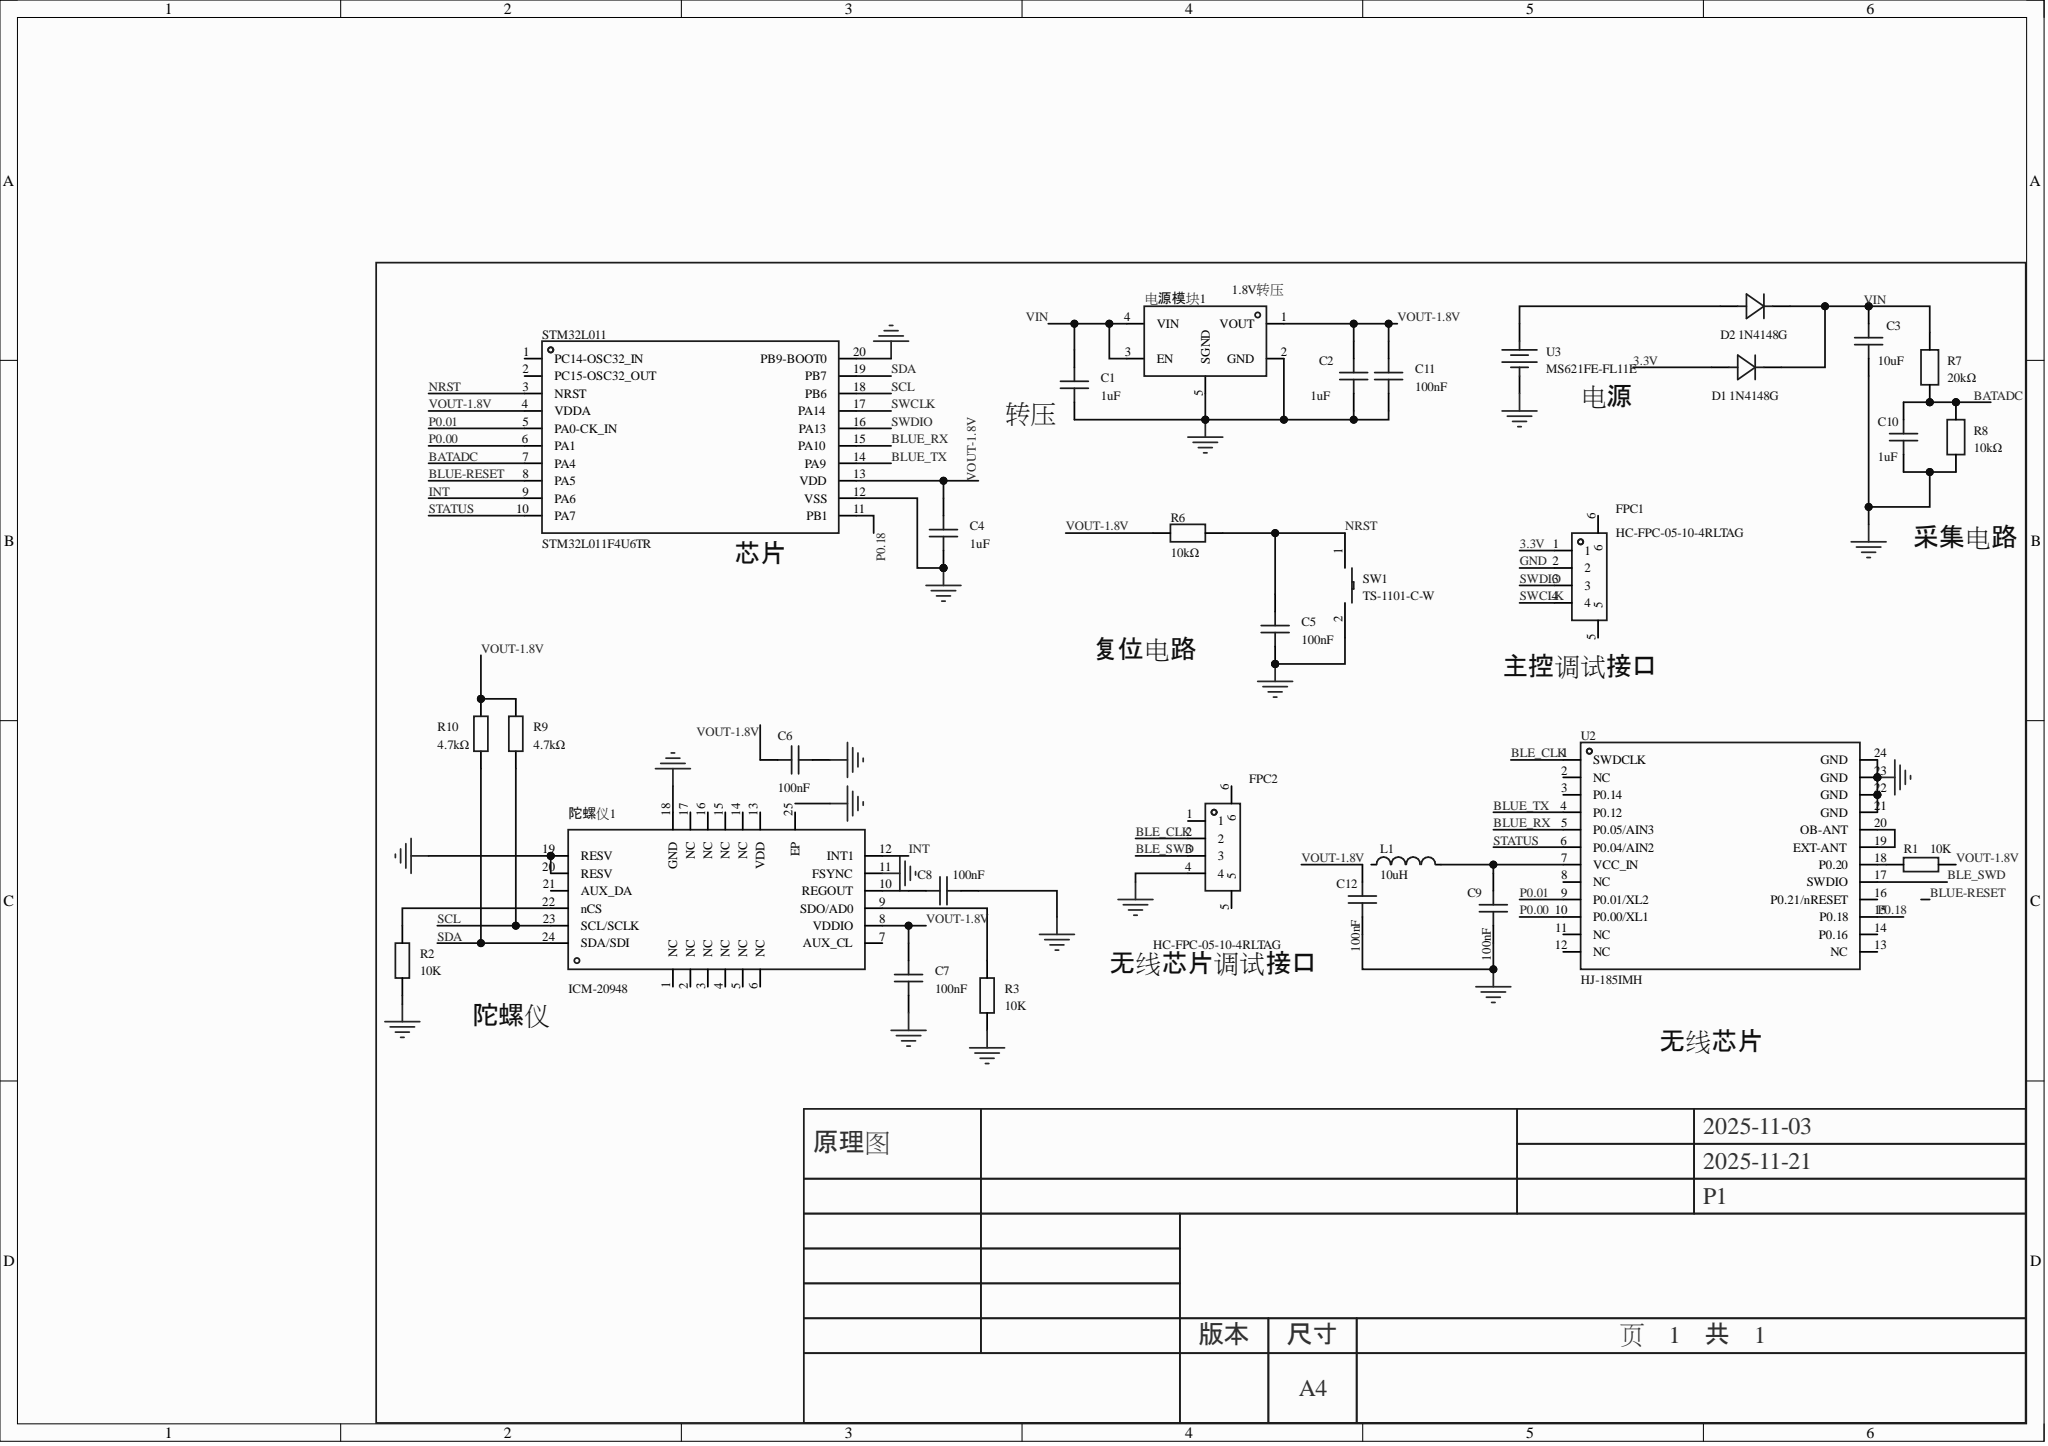Circuit board | Altium Designer | 31 parts | 26 nets
Bill of materials:
Comment,Description,Designator,Footprint,LibRef,Quantity
"1uF","容值:1uF;精度:±10%;额定电压:25V;温度系数:X5R;","C1, C2, C4, C10","C0402","CL05A105KA5NQNC","4"
"10uF","容值:10uF;精度:±10%;额定电压:50V;温度系数:X5R;","C3","C0805","CGA0805X5R106K500MT","1"
"100nF","","C5, C6, C7, C8, C9, C12","C0402","CL05B104KB54PNC, CL05B104KO5NNNC","6"
"100nF","容值:100nF;精度:±10%;额定电压:50V;温度系数:X7R;","C11","C0603","CGA0603X7R104K500JT","1"
"1N4148G","正向压降(Vf):1.25V@150mA;直流反向耐压(Vr):100V;整流电流:150mA;反向恢复时间(Trr):4ns;","D1, D2","SOD-723_L1.0-W0.6-P1.4-RD","1N4148G","2"
"HC-FPC-05-10-4RLTAG","锁定特性:翻盖式;触点类型:下接;触点数量:4P;间距:0.5mm;安装方式:卧贴;工作温度:-55℃~+85℃;","FPC1, FPC2","FPC-SMD_4P-P0.50_HCTL_HC-FPC-05-10-4RLTAG","HC-FPC-05-10-4RLTAG","2"
"10uH","","L1","L0603","L_0603","1"
"10K","","R1, R2, R3","R0603","Res_0603","3"
"10kΩ","","R6, R8","R0402","AS0210KF","2"
"20kΩ","","R7","R0402","FRQ0402F2002TS","1"
"4.7kΩ","","R9, R10","R0402","0402WGF4701TCE","2"
"STM32L011F4U6TR","CPU内核:ARM-M系列;CPU最大主频:32MHz;应用领域:-;","STM32L011","QFN-20_L3.0-W3.0-P0.50-BL","STM32L011F4U6TR","1"
"TS-1101-C-W","电路结构:单刀单掷;按钮形状:矩形按钮;作用力:260gf;安装方式:立贴;开关长度:6mm;开关宽度:3.6mm;开关高度:2.5mm;带支架:不带;触点电流:50mA;额定电压(AC):-;额定电压(DC):12V;额定功率:-;绝缘电阻:-;带灯:无;机械寿命:5万次;","SW1","SW-SMD_L6.0-W3.3-LS8.0","TS-1101-C-W","1"
"HJ-185IMH","","U2","LGA-24_L5.5-W5.0-P0.75-BL-EP","HJ-185IMH","1"
"MS621FE-FL11E","标称电压:3V;","U3","BAT-SMD_FL11E","MS621FE-FL11E","1"
"1.8V转压","输出类型:固定;工作电压:5.5V;输出电压:1.8V;输出电流:250mA;电源纹波抑制比(PSRR):75dB@(1kHz);输出极性:正极;","电源模块1","ZQFN-4L_L1.0-W1.0-P0.63-BL-EP","RT9073A-18GQZ","1"
"ICM-20948","传感器类型:加速度计陀螺仪;接口类型:I2C；SPI;","陀螺仪1","QFN-24_L3.0-W3.0-P0.40-BL-EP","ICM-20948","1"
Netlist (Protel format):
[
C1
C0402
1uF



]
[
C2
C0402
1uF



]
[
C3
C0805
10uF



]
[
C4
C0402
1uF



]
[
C5
C0402
100nF



]
[
C6
C0402
100nF



]
[
C7
C0402
100nF



]
[
C8
C0402
100nF



]
[
C9
C0402
100nF



]
[
C10
C0402
1uF



]
[
C11
C0603
100nF



]
[
C12
C0402
100nF



]
[
D1
SOD-723_L1.0-W0.6-P1.4-RD
1N4148G



]
[
D2
SOD-723_L1.0-W0.6-P1.4-RD
1N4148G



]
[
FPC1
FPC-SMD_4P-P0.50_HCTL_HC-FPC-05-10-4RLTAG
HC-FPC-05-10-4RLTAG



]
[
FPC2
FPC-SMD_4P-P0.50_HCTL_HC-FPC-05-10-4RLTAG
HC-FPC-05-10-4RLTAG



]
[
L1
L0603
10uH



]
[
R1
R0603
10K



]
[
R2
R0603
10K



]
[
R3
R0603
10K



]
[
R6
R0402
10kΩ



]
[
R7
R0402
20kΩ



]
[
R8
R0402
10kΩ



]
[
R9
R0402
4.7kΩ



]
[
R10
R0402
4.7kΩ



]
[
STM32L011
QFN-20_L3.0-W3.0-P0.50-BL
STM32L011F4U6TR



]
[
SW1
SW-SMD_L6.0-W3.3-LS8.0
TS-1101-C-W



]
[
U2
LGA-24_L5.5-W5.0-P0.75-BL-EP
HJ-185IMH



]
[
U3
BAT-SMD_FL11E
MS621FE-FL11E



]
[
电源模块1
ZQFN-4L_L1.0-W1.0-P0.63-BL-EP
1.8V转压



]
[
陀螺仪1
QFN-24_L3.0-W3.0-P0.40-BL-EP
ICM-20948



]
(
VOUT-1.8V
C2-2
C4-2
C6-2
C7-2
C11-2
C12-2
R1-2
R6-1
R9-1
R10-1
STM32L011-4
STM32L011-13
电源模块1-1
陀螺仪1-8
)
(
VIN
C1-2
C3-2
D1-1
D2-1
R7-2
电源模块1-3
电源模块1-4
)
(
SWDIO
FPC1-3
STM32L011-16
)
(
SWCLK
FPC1-4
STM32L011-17
)
(
STATUS
STM32L011-10
U2-6
)
(
SDA
R10-2
STM32L011-19
陀螺仪1-24
)
(
SCL
R9-2
STM32L011-18
陀螺仪1-23
)
(
P0.18
STM32L011-11
U2-15
)
(
P0.01
STM32L011-5
U2-9
)
(
P0.00
STM32L011-6
U2-10
)
(
NRST
C5-2
R6-2
STM32L011-3
SW1-1
)
(
NetU2_19
U2-19
U2-20
)
(
NetR3_2
R3-2
陀螺仪1-9
)
(
NetR2_2
R2-2
陀螺仪1-22
)
(
NetR1_1
R1-1
U2-18
)
(
NetD2_2
D2-2
U3-1
)
(
NetC9_2
C9-2
L1-2
U2-7
)
(
NetC8_1
C8-1
陀螺仪1-10
)
(
INT
STM32L011-9
陀螺仪1-12
)
(
GND
C1-1
C2-1
C3-1
C4-1
C5-1
C6-1
C7-1
C8-2
C9-1
C10-1
C11-1
C12-1
FPC1-2
FPC2-4
R2-1
R3-1
R8-1
STM32L011-12
STM32L011-20
SW1-2
U2-21
U2-22
U2-23
U2-24
U3-2
电源模块1-2
电源模块1-5
陀螺仪1-11
陀螺仪1-18
陀螺仪1-19
陀螺仪1-20
)
(
BLUE_TX
STM32L011-14
U2-4
)
(
BLUE_RX
STM32L011-15
U2-5
)
(
BLE_SWD
FPC2-3
U2-17
)
(
BLE_CLK
FPC2-2
U2-1
)
(
BATADC
C10-2
R7-1
R8-2
STM32L011-7
)
(
3.3V
D1-2
FPC1-1
)